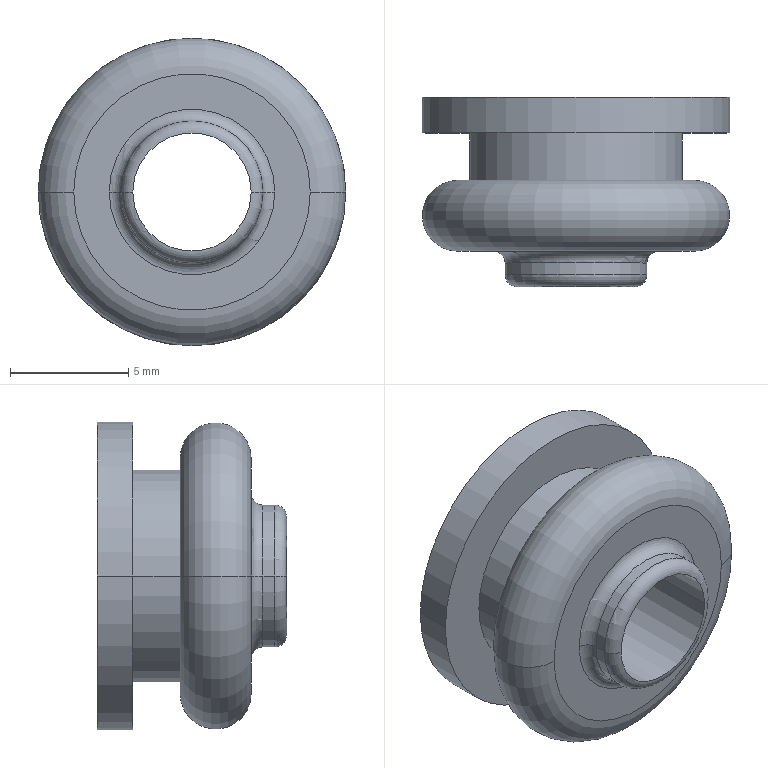Part | STEP file | 233_07_060_230 | 1 solid | 18 faces | box 13 x 8 x 13 mm | volume 572.53 mm3 | cylinder 8 | torus 6 | plane 4 | commonest cylinder face diameters 5 x2 6 x2 9 x2 13 x2
STEP:
#1=CARTESIAN_POINT('',(0.,0.,0.));
#2=DIRECTION('',(0.,0.,1.));
#3=DIRECTION('',(1.,0.,0.));
#4=AXIS2_PLACEMENT_3D('',#1,#2,#3);
#5=CARTESIAN_POINT('',(-2.5,0.,0.));
#6=VERTEX_POINT('',#5);
#7=CARTESIAN_POINT('',(-2.5,-8.,0.));
#8=VERTEX_POINT('',#7);
#9=CARTESIAN_POINT('',(-2.5,0.,0.));
#10=DIRECTION('',(0.,-1.,0.));
#11=VECTOR('',#10,1.);
#12=LINE('',#9,#11);
#13=CARTESIAN_POINT('',(0.,0.4,0.));
#14=DIRECTION('',(0.,-1.,0.));
#15=DIRECTION('',(1.,0.,0.));
#16=AXIS2_PLACEMENT_3D('',#13,#14,#15);
#17=CYLINDRICAL_SURFACE('',#16,2.5);
#18=CARTESIAN_POINT('',(3.142,0.4));
#19=DIRECTION('',(0.,1.));
#20=VECTOR('',#19,1.);
#21=LINE('',#18,#20);
#22=(GEOMETRIC_REPRESENTATION_CONTEXT(2)PARAMETRIC_REPRESENTATION_CONTEXT()REPRESENTATION_CONTEXT('',''));
#23=DEFINITIONAL_REPRESENTATION('',(#21),#22);
#24=PCURVE('',#17,#23);
#25=CARTESIAN_POINT('',(0.,0.4,0.));
#26=DIRECTION('',(0.,-1.,0.));
#27=DIRECTION('',(1.,0.,0.));
#28=AXIS2_PLACEMENT_3D('',#25,#26,#27);
#29=CYLINDRICAL_SURFACE('',#28,2.5);
#30=CARTESIAN_POINT('',(3.142,0.4));
#31=DIRECTION('',(0.,1.));
#32=VECTOR('',#31,1.);
#33=LINE('',#30,#32);
#34=(GEOMETRIC_REPRESENTATION_CONTEXT(2)PARAMETRIC_REPRESENTATION_CONTEXT()REPRESENTATION_CONTEXT('',''));
#35=DEFINITIONAL_REPRESENTATION('',(#33),#34);
#36=PCURVE('',#29,#35);
#37=SURFACE_CURVE('',#12,(#24,#36),.PCURVE_S1.);
#38=EDGE_CURVE('',#6,#8,#37,.T.);
#39=ORIENTED_EDGE('',*,*,#38,.F.);
#40=CARTESIAN_POINT('',(2.5,0.,0.));
#41=VERTEX_POINT('',#40);
#42=CARTESIAN_POINT('',(0.,0.,0.));
#43=DIRECTION('',(0.,-1.,0.));
#44=DIRECTION('',(-1.,0.,0.));
#45=AXIS2_PLACEMENT_3D('',#42,#43,#44);
#46=CIRCLE('',#45,2.5);
#47=CARTESIAN_POINT('',(3.142,0.4));
#48=DIRECTION('',(1.,0.));
#49=VECTOR('',#48,1.);
#50=LINE('',#47,#49);
#51=(GEOMETRIC_REPRESENTATION_CONTEXT(2)PARAMETRIC_REPRESENTATION_CONTEXT()REPRESENTATION_CONTEXT('',''));
#52=DEFINITIONAL_REPRESENTATION('',(#50),#51);
#53=PCURVE('',#17,#52);
#54=CARTESIAN_POINT('',(0.,0.,0.));
#55=DIRECTION('',(0.,-1.,0.));
#56=DIRECTION('',(1.,0.,0.));
#57=AXIS2_PLACEMENT_3D('',#54,#55,#56);
#58=PLANE('',#57);
#59=CARTESIAN_POINT('',(0.,0.));
#60=DIRECTION('',(-1.,0.));
#61=AXIS2_PLACEMENT_2D('',#59,#60);
#62=CIRCLE('',#61,2.5);
#63=(GEOMETRIC_REPRESENTATION_CONTEXT(2)PARAMETRIC_REPRESENTATION_CONTEXT()REPRESENTATION_CONTEXT('',''));
#64=DEFINITIONAL_REPRESENTATION('',(#62),#63);
#65=PCURVE('',#58,#64);
#66=SURFACE_CURVE('',#46,(#53,#65),.PCURVE_S1.);
#67=EDGE_CURVE('',#6,#41,#66,.T.);
#68=ORIENTED_EDGE('',*,*,#67,.T.);
#69=CARTESIAN_POINT('',(2.5,-8.,0.));
#70=VERTEX_POINT('',#69);
#71=CARTESIAN_POINT('',(2.5,0.,0.));
#72=DIRECTION('',(0.,-1.,0.));
#73=VECTOR('',#72,1.);
#74=LINE('',#71,#73);
#75=CARTESIAN_POINT('',(6.283,0.4));
#76=DIRECTION('',(0.,1.));
#77=VECTOR('',#76,1.);
#78=LINE('',#75,#77);
#79=(GEOMETRIC_REPRESENTATION_CONTEXT(2)PARAMETRIC_REPRESENTATION_CONTEXT()REPRESENTATION_CONTEXT('',''));
#80=DEFINITIONAL_REPRESENTATION('',(#78),#79);
#81=PCURVE('',#17,#80);
#82=CARTESIAN_POINT('',(0.,0.4));
#83=DIRECTION('',(0.,1.));
#84=VECTOR('',#83,1.);
#85=LINE('',#82,#84);
#86=(GEOMETRIC_REPRESENTATION_CONTEXT(2)PARAMETRIC_REPRESENTATION_CONTEXT()REPRESENTATION_CONTEXT('',''));
#87=DEFINITIONAL_REPRESENTATION('',(#85),#86);
#88=PCURVE('',#29,#87);
#89=SURFACE_CURVE('',#74,(#81,#88),.PCURVE_S1.);
#90=EDGE_CURVE('',#41,#70,#89,.T.);
#91=ORIENTED_EDGE('',*,*,#90,.T.);
#92=CARTESIAN_POINT('',(0.,-8.,0.));
#93=DIRECTION('',(0.,-1.,0.));
#94=DIRECTION('',(-1.,0.,0.));
#95=AXIS2_PLACEMENT_3D('',#92,#93,#94);
#96=CIRCLE('',#95,2.5);
#97=CARTESIAN_POINT('',(3.142,8.4));
#98=DIRECTION('',(1.,0.));
#99=VECTOR('',#98,1.);
#100=LINE('',#97,#99);
#101=(GEOMETRIC_REPRESENTATION_CONTEXT(2)PARAMETRIC_REPRESENTATION_CONTEXT()REPRESENTATION_CONTEXT('',''));
#102=DEFINITIONAL_REPRESENTATION('',(#100),#101);
#103=PCURVE('',#17,#102);
#104=CARTESIAN_POINT('',(0.,-7.5,0.));
#105=DIRECTION('',(0.,-1.,0.));
#106=DIRECTION('',(1.,0.,0.));
#107=AXIS2_PLACEMENT_3D('',#104,#105,#106);
#108=TOROIDAL_SURFACE('',#107,2.5,0.5);
#109=CARTESIAN_POINT('',(3.142,1.571));
#110=DIRECTION('',(1.,0.));
#111=VECTOR('',#110,1.);
#112=LINE('',#109,#111);
#113=(GEOMETRIC_REPRESENTATION_CONTEXT(2)PARAMETRIC_REPRESENTATION_CONTEXT()REPRESENTATION_CONTEXT('',''));
#114=DEFINITIONAL_REPRESENTATION('',(#112),#113);
#115=PCURVE('',#108,#114);
#116=SURFACE_CURVE('',#96,(#103,#115),.PCURVE_S1.);
#117=EDGE_CURVE('',#8,#70,#116,.T.);
#118=ORIENTED_EDGE('',*,*,#117,.F.);
#119=EDGE_LOOP('',(#39,#68,#91,#118));
#120=FACE_BOUND('',#119,.F.);
#121=ADVANCED_FACE('',(#120),#17,.F.);
#122=ORIENTED_EDGE('',*,*,#38,.T.);
#123=CARTESIAN_POINT('',(0.,-8.,0.));
#124=DIRECTION('',(0.,1.,0.));
#125=DIRECTION('',(-1.,0.,0.));
#126=AXIS2_PLACEMENT_3D('',#123,#124,#125);
#127=CIRCLE('',#126,2.5);
#128=CARTESIAN_POINT('',(3.142,8.4));
#129=DIRECTION('',(-1.,0.));
#130=VECTOR('',#129,1.);
#131=LINE('',#128,#130);
#132=(GEOMETRIC_REPRESENTATION_CONTEXT(2)PARAMETRIC_REPRESENTATION_CONTEXT()REPRESENTATION_CONTEXT('',''));
#133=DEFINITIONAL_REPRESENTATION('',(#131),#132);
#134=PCURVE('',#29,#133);
#135=CARTESIAN_POINT('',(0.,-7.5,0.));
#136=DIRECTION('',(0.,-1.,0.));
#137=DIRECTION('',(1.,0.,0.));
#138=AXIS2_PLACEMENT_3D('',#135,#136,#137);
#139=TOROIDAL_SURFACE('',#138,2.5,0.5);
#140=CARTESIAN_POINT('',(3.142,1.571));
#141=DIRECTION('',(-1.,0.));
#142=VECTOR('',#141,1.);
#143=LINE('',#140,#142);
#144=(GEOMETRIC_REPRESENTATION_CONTEXT(2)PARAMETRIC_REPRESENTATION_CONTEXT()REPRESENTATION_CONTEXT('',''));
#145=DEFINITIONAL_REPRESENTATION('',(#143),#144);
#146=PCURVE('',#139,#145);
#147=SURFACE_CURVE('',#127,(#134,#146),.PCURVE_S1.);
#148=EDGE_CURVE('',#8,#70,#147,.T.);
#149=ORIENTED_EDGE('',*,*,#148,.T.);
#150=ORIENTED_EDGE('',*,*,#90,.F.);
#151=CARTESIAN_POINT('',(0.,0.,0.));
#152=DIRECTION('',(0.,1.,0.));
#153=DIRECTION('',(-1.,0.,0.));
#154=AXIS2_PLACEMENT_3D('',#151,#152,#153);
#155=CIRCLE('',#154,2.5);
#156=CARTESIAN_POINT('',(3.142,0.4));
#157=DIRECTION('',(-1.,0.));
#158=VECTOR('',#157,1.);
#159=LINE('',#156,#158);
#160=(GEOMETRIC_REPRESENTATION_CONTEXT(2)PARAMETRIC_REPRESENTATION_CONTEXT()REPRESENTATION_CONTEXT('',''));
#161=DEFINITIONAL_REPRESENTATION('',(#159),#160);
#162=PCURVE('',#29,#161);
#163=CARTESIAN_POINT('',(-2.5,0.));
#164=CARTESIAN_POINT('',(-2.5,4.33));
#165=CARTESIAN_POINT('',(1.25,2.165));
#166=CARTESIAN_POINT('',(5.,0.));
#167=CARTESIAN_POINT('',(1.25,-2.165));
#168=CARTESIAN_POINT('',(-2.5,-4.33));
#169=CARTESIAN_POINT('',(-2.5,0.));
#170=(BOUNDED_CURVE()B_SPLINE_CURVE(2,(#163,#164,#165,#166,#167,#168,#169),.UNSPECIFIED.,.T.,.F.)B_SPLINE_CURVE_WITH_KNOTS((1,2,2,2,2,1),(-2.094,0.,2.094,4.189,6.283,8.378),.UNSPECIFIED.)CURVE()GEOMETRIC_REPRESENTATION_ITEM()RATIONAL_B_SPLINE_CURVE((1.,0.5,1.,0.5,1.,0.5,1.))REPRESENTATION_ITEM(''));
#171=(GEOMETRIC_REPRESENTATION_CONTEXT(2)PARAMETRIC_REPRESENTATION_CONTEXT()REPRESENTATION_CONTEXT('',''));
#172=DEFINITIONAL_REPRESENTATION('',(#170),#171);
#173=PCURVE('',#58,#172);
#174=SURFACE_CURVE('',#155,(#162,#173),.PCURVE_S1.);
#175=EDGE_CURVE('',#6,#41,#174,.T.);
#176=ORIENTED_EDGE('',*,*,#175,.F.);
#177=EDGE_LOOP('',(#122,#149,#150,#176));
#178=FACE_BOUND('',#177,.F.);
#179=ADVANCED_FACE('',(#178),#29,.F.);
#180=ORIENTED_EDGE('',*,*,#148,.T.);
#181=CARTESIAN_POINT('',(3.,-7.5,0.));
#182=VERTEX_POINT('',#181);
#183=CARTESIAN_POINT('',(2.5,-7.5,0.));
#184=DIRECTION('',(0.,0.,1.));
#185=DIRECTION('',(0.,-1.,0.));
#186=AXIS2_PLACEMENT_3D('',#183,#184,#185);
#187=CIRCLE('',#186,0.5);
#188=CARTESIAN_POINT('',(0.,1.571));
#189=DIRECTION('',(0.,-1.));
#190=VECTOR('',#189,1.);
#191=LINE('',#188,#190);
#192=(GEOMETRIC_REPRESENTATION_CONTEXT(2)PARAMETRIC_REPRESENTATION_CONTEXT()REPRESENTATION_CONTEXT('',''));
#193=DEFINITIONAL_REPRESENTATION('',(#191),#192);
#194=PCURVE('',#139,#193);
#195=CARTESIAN_POINT('',(6.283,1.571));
#196=DIRECTION('',(0.,-1.));
#197=VECTOR('',#196,1.);
#198=LINE('',#195,#197);
#199=(GEOMETRIC_REPRESENTATION_CONTEXT(2)PARAMETRIC_REPRESENTATION_CONTEXT()REPRESENTATION_CONTEXT('',''));
#200=DEFINITIONAL_REPRESENTATION('',(#198),#199);
#201=PCURVE('',#108,#200);
#202=SURFACE_CURVE('',#187,(#194,#201),.PCURVE_S1.);
#203=EDGE_CURVE('',#70,#182,#202,.T.);
#204=ORIENTED_EDGE('',*,*,#203,.T.);
#205=CARTESIAN_POINT('',(-3.,-7.5,0.));
#206=VERTEX_POINT('',#205);
#207=CARTESIAN_POINT('',(0.,-7.5,0.));
#208=DIRECTION('',(0.,1.,0.));
#209=DIRECTION('',(-1.,0.,0.));
#210=AXIS2_PLACEMENT_3D('',#207,#208,#209);
#211=CIRCLE('',#210,3.);
#212=CARTESIAN_POINT('',(3.142,0.));
#213=DIRECTION('',(-1.,0.));
#214=VECTOR('',#213,1.);
#215=LINE('',#212,#214);
#216=(GEOMETRIC_REPRESENTATION_CONTEXT(2)PARAMETRIC_REPRESENTATION_CONTEXT()REPRESENTATION_CONTEXT('',''));
#217=DEFINITIONAL_REPRESENTATION('',(#215),#216);
#218=PCURVE('',#139,#217);
#219=CARTESIAN_POINT('',(0.,0.4,0.));
#220=DIRECTION('',(0.,-1.,0.));
#221=DIRECTION('',(1.,0.,0.));
#222=AXIS2_PLACEMENT_3D('',#219,#220,#221);
#223=CYLINDRICAL_SURFACE('',#222,3.);
#224=CARTESIAN_POINT('',(3.142,7.9));
#225=DIRECTION('',(-1.,0.));
#226=VECTOR('',#225,1.);
#227=LINE('',#224,#226);
#228=(GEOMETRIC_REPRESENTATION_CONTEXT(2)PARAMETRIC_REPRESENTATION_CONTEXT()REPRESENTATION_CONTEXT('',''));
#229=DEFINITIONAL_REPRESENTATION('',(#227),#228);
#230=PCURVE('',#223,#229);
#231=SURFACE_CURVE('',#211,(#218,#230),.PCURVE_S1.);
#232=EDGE_CURVE('',#206,#182,#231,.T.);
#233=ORIENTED_EDGE('',*,*,#232,.F.);
#234=CARTESIAN_POINT('',(-2.5,-7.5,0.));
#235=DIRECTION('',(0.,0.,-1.));
#236=DIRECTION('',(0.,-1.,0.));
#237=AXIS2_PLACEMENT_3D('',#234,#235,#236);
#238=CIRCLE('',#237,0.5);
#239=CARTESIAN_POINT('',(3.142,1.571));
#240=DIRECTION('',(0.,-1.));
#241=VECTOR('',#240,1.);
#242=LINE('',#239,#241);
#243=(GEOMETRIC_REPRESENTATION_CONTEXT(2)PARAMETRIC_REPRESENTATION_CONTEXT()REPRESENTATION_CONTEXT('',''));
#244=DEFINITIONAL_REPRESENTATION('',(#242),#243);
#245=PCURVE('',#139,#244);
#246=CARTESIAN_POINT('',(3.142,1.571));
#247=DIRECTION('',(0.,-1.));
#248=VECTOR('',#247,1.);
#249=LINE('',#246,#248);
#250=(GEOMETRIC_REPRESENTATION_CONTEXT(2)PARAMETRIC_REPRESENTATION_CONTEXT()REPRESENTATION_CONTEXT('',''));
#251=DEFINITIONAL_REPRESENTATION('',(#249),#250);
#252=PCURVE('',#108,#251);
#253=SURFACE_CURVE('',#238,(#245,#252),.PCURVE_S1.);
#254=EDGE_CURVE('',#8,#206,#253,.T.);
#255=ORIENTED_EDGE('',*,*,#254,.F.);
#256=EDGE_LOOP('',(#180,#204,#233,#255));
#257=FACE_BOUND('',#256,.T.);
#258=ADVANCED_FACE('',(#257),#139,.T.);
#259=CARTESIAN_POINT('',(0.,-7.5,0.));
#260=DIRECTION('',(0.,-1.,0.));
#261=DIRECTION('',(-1.,0.,0.));
#262=AXIS2_PLACEMENT_3D('',#259,#260,#261);
#263=CIRCLE('',#262,3.);
#264=CARTESIAN_POINT('',(3.142,0.));
#265=DIRECTION('',(1.,0.));
#266=VECTOR('',#265,1.);
#267=LINE('',#264,#266);
#268=(GEOMETRIC_REPRESENTATION_CONTEXT(2)PARAMETRIC_REPRESENTATION_CONTEXT()REPRESENTATION_CONTEXT('',''));
#269=DEFINITIONAL_REPRESENTATION('',(#267),#268);
#270=PCURVE('',#108,#269);
#271=CARTESIAN_POINT('',(0.,0.4,0.));
#272=DIRECTION('',(0.,-1.,0.));
#273=DIRECTION('',(1.,0.,0.));
#274=AXIS2_PLACEMENT_3D('',#271,#272,#273);
#275=CYLINDRICAL_SURFACE('',#274,3.);
#276=CARTESIAN_POINT('',(3.142,7.9));
#277=DIRECTION('',(1.,0.));
#278=VECTOR('',#277,1.);
#279=LINE('',#276,#278);
#280=(GEOMETRIC_REPRESENTATION_CONTEXT(2)PARAMETRIC_REPRESENTATION_CONTEXT()REPRESENTATION_CONTEXT('',''));
#281=DEFINITIONAL_REPRESENTATION('',(#279),#280);
#282=PCURVE('',#275,#281);
#283=SURFACE_CURVE('',#263,(#270,#282),.PCURVE_S1.);
#284=EDGE_CURVE('',#206,#182,#283,.T.);
#285=ORIENTED_EDGE('',*,*,#284,.T.);
#286=ORIENTED_EDGE('',*,*,#203,.F.);
#287=ORIENTED_EDGE('',*,*,#117,.F.);
#288=ORIENTED_EDGE('',*,*,#254,.T.);
#289=EDGE_LOOP('',(#285,#286,#287,#288));
#290=FACE_BOUND('',#289,.T.);
#291=ADVANCED_FACE('',(#290),#108,.T.);
#292=CARTESIAN_POINT('',(-3.,-7.,0.));
#293=VERTEX_POINT('',#292);
#294=CARTESIAN_POINT('',(3.,-7.,0.));
#295=VERTEX_POINT('',#294);
#296=CARTESIAN_POINT('',(0.,-7.,0.));
#297=DIRECTION('',(0.,-1.,0.));
#298=DIRECTION('',(-1.,0.,0.));
#299=AXIS2_PLACEMENT_3D('',#296,#297,#298);
#300=CIRCLE('',#299,3.);
#301=CARTESIAN_POINT('',(3.142,7.4));
#302=DIRECTION('',(1.,0.));
#303=VECTOR('',#302,1.);
#304=LINE('',#301,#303);
#305=(GEOMETRIC_REPRESENTATION_CONTEXT(2)PARAMETRIC_REPRESENTATION_CONTEXT()REPRESENTATION_CONTEXT('',''));
#306=DEFINITIONAL_REPRESENTATION('',(#304),#305);
#307=PCURVE('',#275,#306);
#308=CARTESIAN_POINT('',(0.,-7.,0.));
#309=DIRECTION('',(0.,-1.,0.));
#310=DIRECTION('',(1.,0.,0.));
#311=AXIS2_PLACEMENT_3D('',#308,#309,#310);
#312=TOROIDAL_SURFACE('',#311,3.5,0.5);
#313=CARTESIAN_POINT('',(3.142,3.142));
#314=DIRECTION('',(1.,0.));
#315=VECTOR('',#314,1.);
#316=LINE('',#313,#315);
#317=(GEOMETRIC_REPRESENTATION_CONTEXT(2)PARAMETRIC_REPRESENTATION_CONTEXT()REPRESENTATION_CONTEXT('',''));
#318=DEFINITIONAL_REPRESENTATION('',(#316),#317);
#319=PCURVE('',#312,#318);
#320=SURFACE_CURVE('',#300,(#307,#319),.PCURVE_S1.);
#321=EDGE_CURVE('',#293,#295,#320,.T.);
#322=ORIENTED_EDGE('',*,*,#321,.T.);
#323=CARTESIAN_POINT('',(3.,-7.5,0.));
#324=DIRECTION('',(0.,1.,0.));
#325=VECTOR('',#324,1.);
#326=LINE('',#323,#325);
#327=CARTESIAN_POINT('',(6.283,7.9));
#328=DIRECTION('',(0.,-1.));
#329=VECTOR('',#328,1.);
#330=LINE('',#327,#329);
#331=(GEOMETRIC_REPRESENTATION_CONTEXT(2)PARAMETRIC_REPRESENTATION_CONTEXT()REPRESENTATION_CONTEXT('',''));
#332=DEFINITIONAL_REPRESENTATION('',(#330),#331);
#333=PCURVE('',#275,#332);
#334=CARTESIAN_POINT('',(0.,7.9));
#335=DIRECTION('',(0.,-1.));
#336=VECTOR('',#335,1.);
#337=LINE('',#334,#336);
#338=(GEOMETRIC_REPRESENTATION_CONTEXT(2)PARAMETRIC_REPRESENTATION_CONTEXT()REPRESENTATION_CONTEXT('',''));
#339=DEFINITIONAL_REPRESENTATION('',(#337),#338);
#340=PCURVE('',#223,#339);
#341=SURFACE_CURVE('',#326,(#333,#340),.PCURVE_S1.);
#342=EDGE_CURVE('',#182,#295,#341,.T.);
#343=ORIENTED_EDGE('',*,*,#342,.F.);
#344=ORIENTED_EDGE('',*,*,#284,.F.);
#345=CARTESIAN_POINT('',(-3.,-7.5,0.));
#346=DIRECTION('',(0.,1.,0.));
#347=VECTOR('',#346,1.);
#348=LINE('',#345,#347);
#349=CARTESIAN_POINT('',(3.142,7.9));
#350=DIRECTION('',(0.,-1.));
#351=VECTOR('',#350,1.);
#352=LINE('',#349,#351);
#353=(GEOMETRIC_REPRESENTATION_CONTEXT(2)PARAMETRIC_REPRESENTATION_CONTEXT()REPRESENTATION_CONTEXT('',''));
#354=DEFINITIONAL_REPRESENTATION('',(#352),#353);
#355=PCURVE('',#275,#354);
#356=CARTESIAN_POINT('',(3.142,7.9));
#357=DIRECTION('',(0.,-1.));
#358=VECTOR('',#357,1.);
#359=LINE('',#356,#358);
#360=(GEOMETRIC_REPRESENTATION_CONTEXT(2)PARAMETRIC_REPRESENTATION_CONTEXT()REPRESENTATION_CONTEXT('',''));
#361=DEFINITIONAL_REPRESENTATION('',(#359),#360);
#362=PCURVE('',#223,#361);
#363=SURFACE_CURVE('',#348,(#355,#362),.PCURVE_S1.);
#364=EDGE_CURVE('',#206,#293,#363,.T.);
#365=ORIENTED_EDGE('',*,*,#364,.T.);
#366=EDGE_LOOP('',(#322,#343,#344,#365));
#367=FACE_BOUND('',#366,.T.);
#368=ADVANCED_FACE('',(#367),#275,.T.);
#369=ORIENTED_EDGE('',*,*,#232,.T.);
#370=ORIENTED_EDGE('',*,*,#342,.T.);
#371=CARTESIAN_POINT('',(0.,-7.,0.));
#372=DIRECTION('',(0.,1.,0.));
#373=DIRECTION('',(-1.,0.,0.));
#374=AXIS2_PLACEMENT_3D('',#371,#372,#373);
#375=CIRCLE('',#374,3.);
#376=CARTESIAN_POINT('',(3.142,7.4));
#377=DIRECTION('',(-1.,0.));
#378=VECTOR('',#377,1.);
#379=LINE('',#376,#378);
#380=(GEOMETRIC_REPRESENTATION_CONTEXT(2)PARAMETRIC_REPRESENTATION_CONTEXT()REPRESENTATION_CONTEXT('',''));
#381=DEFINITIONAL_REPRESENTATION('',(#379),#380);
#382=PCURVE('',#223,#381);
#383=CARTESIAN_POINT('',(0.,-7.,0.));
#384=DIRECTION('',(0.,-1.,0.));
#385=DIRECTION('',(1.,0.,0.));
#386=AXIS2_PLACEMENT_3D('',#383,#384,#385);
#387=TOROIDAL_SURFACE('',#386,3.5,0.5);
#388=CARTESIAN_POINT('',(3.142,3.142));
#389=DIRECTION('',(-1.,0.));
#390=VECTOR('',#389,1.);
#391=LINE('',#388,#390);
#392=(GEOMETRIC_REPRESENTATION_CONTEXT(2)PARAMETRIC_REPRESENTATION_CONTEXT()REPRESENTATION_CONTEXT('',''));
#393=DEFINITIONAL_REPRESENTATION('',(#391),#392);
#394=PCURVE('',#387,#393);
#395=SURFACE_CURVE('',#375,(#382,#394),.PCURVE_S1.);
#396=EDGE_CURVE('',#293,#295,#395,.T.);
#397=ORIENTED_EDGE('',*,*,#396,.F.);
#398=ORIENTED_EDGE('',*,*,#364,.F.);
#399=EDGE_LOOP('',(#369,#370,#397,#398));
#400=FACE_BOUND('',#399,.T.);
#401=ADVANCED_FACE('',(#400),#223,.T.);
#402=CARTESIAN_POINT('',(-3.5,-6.5,0.));
#403=VERTEX_POINT('',#402);
#404=CARTESIAN_POINT('',(-3.5,-7.,0.));
#405=DIRECTION('',(0.,0.,1.));
#406=DIRECTION('',(1.,0.,0.));
#407=AXIS2_PLACEMENT_3D('',#404,#405,#406);
#408=CIRCLE('',#407,0.5);
#409=CARTESIAN_POINT('',(3.142,3.142));
#410=DIRECTION('',(0.,1.));
#411=VECTOR('',#410,1.);
#412=LINE('',#409,#411);
#413=(GEOMETRIC_REPRESENTATION_CONTEXT(2)PARAMETRIC_REPRESENTATION_CONTEXT()REPRESENTATION_CONTEXT('',''));
#414=DEFINITIONAL_REPRESENTATION('',(#412),#413);
#415=PCURVE('',#387,#414);
#416=CARTESIAN_POINT('',(3.142,3.142));
#417=DIRECTION('',(0.,1.));
#418=VECTOR('',#417,1.);
#419=LINE('',#416,#418);
#420=(GEOMETRIC_REPRESENTATION_CONTEXT(2)PARAMETRIC_REPRESENTATION_CONTEXT()REPRESENTATION_CONTEXT('',''));
#421=DEFINITIONAL_REPRESENTATION('',(#419),#420);
#422=PCURVE('',#312,#421);
#423=SURFACE_CURVE('',#408,(#415,#422),.PCURVE_S1.);
#424=EDGE_CURVE('',#293,#403,#423,.T.);
#425=ORIENTED_EDGE('',*,*,#424,.T.);
#426=CARTESIAN_POINT('',(3.5,-6.5,0.));
#427=VERTEX_POINT('',#426);
#428=CARTESIAN_POINT('',(0.,-6.5,0.));
#429=DIRECTION('',(0.,1.,0.));
#430=DIRECTION('',(-1.,0.,0.));
#431=AXIS2_PLACEMENT_3D('',#428,#429,#430);
#432=CIRCLE('',#431,3.5);
#433=CARTESIAN_POINT('',(3.142,4.712));
#434=DIRECTION('',(-1.,0.));
#435=VECTOR('',#434,1.);
#436=LINE('',#433,#435);
#437=(GEOMETRIC_REPRESENTATION_CONTEXT(2)PARAMETRIC_REPRESENTATION_CONTEXT()REPRESENTATION_CONTEXT('',''));
#438=DEFINITIONAL_REPRESENTATION('',(#436),#437);
#439=PCURVE('',#387,#438);
#440=CARTESIAN_POINT('',(0.,-6.5,0.));
#441=DIRECTION('',(0.,-1.,0.));
#442=DIRECTION('',(1.,0.,0.));
#443=AXIS2_PLACEMENT_3D('',#440,#441,#442);
#444=PLANE('',#443);
#445=CARTESIAN_POINT('',(-3.5,0.));
#446=CARTESIAN_POINT('',(-3.5,6.062));
#447=CARTESIAN_POINT('',(1.75,3.031));
#448=CARTESIAN_POINT('',(7.,0.));
#449=CARTESIAN_POINT('',(1.75,-3.031));
#450=CARTESIAN_POINT('',(-3.5,-6.062));
#451=CARTESIAN_POINT('',(-3.5,0.));
#452=(BOUNDED_CURVE()B_SPLINE_CURVE(2,(#445,#446,#447,#448,#449,#450,#451),.UNSPECIFIED.,.T.,.F.)B_SPLINE_CURVE_WITH_KNOTS((1,2,2,2,2,1),(-2.094,0.,2.094,4.189,6.283,8.378),.UNSPECIFIED.)CURVE()GEOMETRIC_REPRESENTATION_ITEM()RATIONAL_B_SPLINE_CURVE((1.,0.5,1.,0.5,1.,0.5,1.))REPRESENTATION_ITEM(''));
#453=(GEOMETRIC_REPRESENTATION_CONTEXT(2)PARAMETRIC_REPRESENTATION_CONTEXT()REPRESENTATION_CONTEXT('',''));
#454=DEFINITIONAL_REPRESENTATION('',(#452),#453);
#455=PCURVE('',#444,#454);
#456=SURFACE_CURVE('',#432,(#439,#455),.PCURVE_S1.);
#457=EDGE_CURVE('',#403,#427,#456,.T.);
#458=ORIENTED_EDGE('',*,*,#457,.T.);
#459=CARTESIAN_POINT('',(3.5,-7.,0.));
#460=DIRECTION('',(0.,0.,-1.));
#461=DIRECTION('',(-1.,0.,0.));
#462=AXIS2_PLACEMENT_3D('',#459,#460,#461);
#463=CIRCLE('',#462,0.5);
#464=CARTESIAN_POINT('',(0.,3.142));
#465=DIRECTION('',(0.,1.));
#466=VECTOR('',#465,1.);
#467=LINE('',#464,#466);
#468=(GEOMETRIC_REPRESENTATION_CONTEXT(2)PARAMETRIC_REPRESENTATION_CONTEXT()REPRESENTATION_CONTEXT('',''));
#469=DEFINITIONAL_REPRESENTATION('',(#467),#468);
#470=PCURVE('',#387,#469);
#471=CARTESIAN_POINT('',(6.283,3.142));
#472=DIRECTION('',(0.,1.));
#473=VECTOR('',#472,1.);
#474=LINE('',#471,#473);
#475=(GEOMETRIC_REPRESENTATION_CONTEXT(2)PARAMETRIC_REPRESENTATION_CONTEXT()REPRESENTATION_CONTEXT('',''));
#476=DEFINITIONAL_REPRESENTATION('',(#474),#475);
#477=PCURVE('',#312,#476);
#478=SURFACE_CURVE('',#463,(#470,#477),.PCURVE_S1.);
#479=EDGE_CURVE('',#295,#427,#478,.T.);
#480=ORIENTED_EDGE('',*,*,#479,.F.);
#481=ORIENTED_EDGE('',*,*,#396,.F.);
#482=EDGE_LOOP('',(#425,#458,#480,#481));
#483=FACE_BOUND('',#482,.F.);
#484=ADVANCED_FACE('',(#483),#387,.F.);
#485=ORIENTED_EDGE('',*,*,#424,.F.);
#486=ORIENTED_EDGE('',*,*,#321,.T.);
#487=ORIENTED_EDGE('',*,*,#479,.T.);
#488=CARTESIAN_POINT('',(0.,-6.5,0.));
#489=DIRECTION('',(0.,-1.,0.));
#490=DIRECTION('',(-1.,0.,0.));
#491=AXIS2_PLACEMENT_3D('',#488,#489,#490);
#492=CIRCLE('',#491,3.5);
#493=CARTESIAN_POINT('',(3.142,4.712));
#494=DIRECTION('',(1.,0.));
#495=VECTOR('',#494,1.);
#496=LINE('',#493,#495);
#497=(GEOMETRIC_REPRESENTATION_CONTEXT(2)PARAMETRIC_REPRESENTATION_CONTEXT()REPRESENTATION_CONTEXT('',''));
#498=DEFINITIONAL_REPRESENTATION('',(#496),#497);
#499=PCURVE('',#312,#498);
#500=CARTESIAN_POINT('',(0.,0.));
#501=DIRECTION('',(-1.,0.));
#502=AXIS2_PLACEMENT_2D('',#500,#501);
#503=CIRCLE('',#502,3.5);
#504=(GEOMETRIC_REPRESENTATION_CONTEXT(2)PARAMETRIC_REPRESENTATION_CONTEXT()REPRESENTATION_CONTEXT('',''));
#505=DEFINITIONAL_REPRESENTATION('',(#503),#504);
#506=PCURVE('',#444,#505);
#507=SURFACE_CURVE('',#492,(#499,#506),.PCURVE_S1.);
#508=EDGE_CURVE('',#403,#427,#507,.T.);
#509=ORIENTED_EDGE('',*,*,#508,.F.);
#510=EDGE_LOOP('',(#485,#486,#487,#509));
#511=FACE_BOUND('',#510,.F.);
#512=ADVANCED_FACE('',(#511),#312,.F.);
#513=CARTESIAN_POINT('',(-5.,-6.5,0.));
#514=VERTEX_POINT('',#513);
#515=CARTESIAN_POINT('',(5.,-6.5,0.));
#516=VERTEX_POINT('',#515);
#517=CARTESIAN_POINT('',(0.,-6.5,0.));
#518=DIRECTION('',(0.,-1.,0.));
#519=DIRECTION('',(-1.,0.,0.));
#520=AXIS2_PLACEMENT_3D('',#517,#518,#519);
#521=CIRCLE('',#520,5.);
#522=CARTESIAN_POINT('',(0.,0.));
#523=DIRECTION('',(-1.,0.));
#524=AXIS2_PLACEMENT_2D('',#522,#523);
#525=CIRCLE('',#524,5.);
#526=(GEOMETRIC_REPRESENTATION_CONTEXT(2)PARAMETRIC_REPRESENTATION_CONTEXT()REPRESENTATION_CONTEXT('',''));
#527=DEFINITIONAL_REPRESENTATION('',(#525),#526);
#528=PCURVE('',#444,#527);
#529=CARTESIAN_POINT('',(0.,-5.,0.));
#530=DIRECTION('',(0.,-1.,0.));
#531=DIRECTION('',(1.,0.,0.));
#532=AXIS2_PLACEMENT_3D('',#529,#530,#531);
#533=TOROIDAL_SURFACE('',#532,5.,1.5);
#534=CARTESIAN_POINT('',(3.142,7.854));
#535=DIRECTION('',(1.,0.));
#536=VECTOR('',#535,1.);
#537=LINE('',#534,#536);
#538=(GEOMETRIC_REPRESENTATION_CONTEXT(2)PARAMETRIC_REPRESENTATION_CONTEXT()REPRESENTATION_CONTEXT('',''));
#539=DEFINITIONAL_REPRESENTATION('',(#537),#538);
#540=PCURVE('',#533,#539);
#541=SURFACE_CURVE('',#521,(#528,#540),.PCURVE_S1.);
#542=EDGE_CURVE('',#514,#516,#541,.T.);
#543=ORIENTED_EDGE('',*,*,#542,.F.);
#544=CARTESIAN_POINT('',(0.,-6.5,0.));
#545=DIRECTION('',(0.,1.,0.));
#546=DIRECTION('',(-1.,0.,0.));
#547=AXIS2_PLACEMENT_3D('',#544,#545,#546);
#548=CIRCLE('',#547,5.);
#549=CARTESIAN_POINT('',(-5.,0.));
#550=CARTESIAN_POINT('',(-5.,8.66));
#551=CARTESIAN_POINT('',(2.5,4.33));
#552=CARTESIAN_POINT('',(10.,0.));
#553=CARTESIAN_POINT('',(2.5,-4.33));
#554=CARTESIAN_POINT('',(-5.,-8.66));
#555=CARTESIAN_POINT('',(-5.,0.));
#556=(BOUNDED_CURVE()B_SPLINE_CURVE(2,(#549,#550,#551,#552,#553,#554,#555),.UNSPECIFIED.,.T.,.F.)B_SPLINE_CURVE_WITH_KNOTS((1,2,2,2,2,1),(-2.094,0.,2.094,4.189,6.283,8.378),.UNSPECIFIED.)CURVE()GEOMETRIC_REPRESENTATION_ITEM()RATIONAL_B_SPLINE_CURVE((1.,0.5,1.,0.5,1.,0.5,1.))REPRESENTATION_ITEM(''));
#557=(GEOMETRIC_REPRESENTATION_CONTEXT(2)PARAMETRIC_REPRESENTATION_CONTEXT()REPRESENTATION_CONTEXT('',''));
#558=DEFINITIONAL_REPRESENTATION('',(#556),#557);
#559=PCURVE('',#444,#558);
#560=CARTESIAN_POINT('',(0.,-5.,0.));
#561=DIRECTION('',(0.,-1.,0.));
#562=DIRECTION('',(1.,0.,0.));
#563=AXIS2_PLACEMENT_3D('',#560,#561,#562);
#564=TOROIDAL_SURFACE('',#563,5.,1.5);
#565=CARTESIAN_POINT('',(3.142,1.571));
#566=DIRECTION('',(-1.,0.));
#567=VECTOR('',#566,1.);
#568=LINE('',#565,#567);
#569=(GEOMETRIC_REPRESENTATION_CONTEXT(2)PARAMETRIC_REPRESENTATION_CONTEXT()REPRESENTATION_CONTEXT('',''));
#570=DEFINITIONAL_REPRESENTATION('',(#568),#569);
#571=PCURVE('',#564,#570);
#572=SURFACE_CURVE('',#548,(#559,#571),.PCURVE_S1.);
#573=EDGE_CURVE('',#514,#516,#572,.T.);
#574=ORIENTED_EDGE('',*,*,#573,.T.);
#575=EDGE_LOOP('',(#543,#574));
#576=FACE_BOUND('',#575,.F.);
#577=ORIENTED_EDGE('',*,*,#457,.F.);
#578=ORIENTED_EDGE('',*,*,#508,.T.);
#579=EDGE_LOOP('',(#577,#578));
#580=FACE_BOUND('',#579,.F.);
#581=ADVANCED_FACE('',(#576,#580),#444,.T.);
#582=CARTESIAN_POINT('',(-5.,-3.5,0.));
#583=VERTEX_POINT('',#582);
#584=CARTESIAN_POINT('',(5.,-3.5,0.));
#585=VERTEX_POINT('',#584);
#586=CARTESIAN_POINT('',(0.,-3.5,0.));
#587=DIRECTION('',(0.,-1.,0.));
#588=DIRECTION('',(-1.,0.,0.));
#589=AXIS2_PLACEMENT_3D('',#586,#587,#588);
#590=CIRCLE('',#589,5.);
#591=CARTESIAN_POINT('',(3.142,4.712));
#592=DIRECTION('',(1.,0.));
#593=VECTOR('',#592,1.);
#594=LINE('',#591,#593);
#595=(GEOMETRIC_REPRESENTATION_CONTEXT(2)PARAMETRIC_REPRESENTATION_CONTEXT()REPRESENTATION_CONTEXT('',''));
#596=DEFINITIONAL_REPRESENTATION('',(#594),#595);
#597=PCURVE('',#533,#596);
#598=CARTESIAN_POINT('',(0.,-3.5,0.));
#599=DIRECTION('',(0.,-1.,0.));
#600=DIRECTION('',(1.,0.,0.));
#601=AXIS2_PLACEMENT_3D('',#598,#599,#600);
#602=PLANE('',#601);
#603=CARTESIAN_POINT('',(0.,0.));
#604=DIRECTION('',(-1.,0.));
#605=AXIS2_PLACEMENT_2D('',#603,#604);
#606=CIRCLE('',#605,5.);
#607=(GEOMETRIC_REPRESENTATION_CONTEXT(2)PARAMETRIC_REPRESENTATION_CONTEXT()REPRESENTATION_CONTEXT('',''));
#608=DEFINITIONAL_REPRESENTATION('',(#606),#607);
#609=PCURVE('',#602,#608);
#610=SURFACE_CURVE('',#590,(#597,#609),.PCURVE_S1.);
#611=EDGE_CURVE('',#583,#585,#610,.T.);
#612=ORIENTED_EDGE('',*,*,#611,.T.);
#613=CARTESIAN_POINT('',(5.,-5.,0.));
#614=DIRECTION('',(0.,0.,1.));
#615=DIRECTION('',(0.,-1.,0.));
#616=AXIS2_PLACEMENT_3D('',#613,#614,#615);
#617=CIRCLE('',#616,1.5);
#618=CARTESIAN_POINT('',(6.283,7.854));
#619=DIRECTION('',(0.,-1.));
#620=VECTOR('',#619,1.);
#621=LINE('',#618,#620);
#622=(GEOMETRIC_REPRESENTATION_CONTEXT(2)PARAMETRIC_REPRESENTATION_CONTEXT()REPRESENTATION_CONTEXT('',''));
#623=DEFINITIONAL_REPRESENTATION('',(#621),#622);
#624=PCURVE('',#533,#623);
#625=CARTESIAN_POINT('',(0.,1.571));
#626=DIRECTION('',(0.,-1.));
#627=VECTOR('',#626,1.);
#628=LINE('',#625,#627);
#629=(GEOMETRIC_REPRESENTATION_CONTEXT(2)PARAMETRIC_REPRESENTATION_CONTEXT()REPRESENTATION_CONTEXT('',''));
#630=DEFINITIONAL_REPRESENTATION('',(#628),#629);
#631=PCURVE('',#564,#630);
#632=SURFACE_CURVE('',#617,(#624,#631),.PCURVE_S1.);
#633=EDGE_CURVE('',#516,#585,#632,.T.);
#634=ORIENTED_EDGE('',*,*,#633,.F.);
#635=ORIENTED_EDGE('',*,*,#542,.F.);
#636=CARTESIAN_POINT('',(-5.,-5.,0.));
#637=DIRECTION('',(0.,0.,-1.));
#638=DIRECTION('',(0.,-1.,0.));
#639=AXIS2_PLACEMENT_3D('',#636,#637,#638);
#640=CIRCLE('',#639,1.5);
#641=CARTESIAN_POINT('',(3.142,7.854));
#642=DIRECTION('',(0.,-1.));
#643=VECTOR('',#642,1.);
#644=LINE('',#641,#643);
#645=(GEOMETRIC_REPRESENTATION_CONTEXT(2)PARAMETRIC_REPRESENTATION_CONTEXT()REPRESENTATION_CONTEXT('',''));
#646=DEFINITIONAL_REPRESENTATION('',(#644),#645);
#647=PCURVE('',#533,#646);
#648=CARTESIAN_POINT('',(3.142,1.571));
#649=DIRECTION('',(0.,-1.));
#650=VECTOR('',#649,1.);
#651=LINE('',#648,#650);
#652=(GEOMETRIC_REPRESENTATION_CONTEXT(2)PARAMETRIC_REPRESENTATION_CONTEXT()REPRESENTATION_CONTEXT('',''));
#653=DEFINITIONAL_REPRESENTATION('',(#651),#652);
#654=PCURVE('',#564,#653);
#655=SURFACE_CURVE('',#640,(#647,#654),.PCURVE_S1.);
#656=EDGE_CURVE('',#514,#583,#655,.T.);
#657=ORIENTED_EDGE('',*,*,#656,.T.);
#658=EDGE_LOOP('',(#612,#634,#635,#657));
#659=FACE_BOUND('',#658,.T.);
#660=ADVANCED_FACE('',(#659),#533,.T.);
#661=ORIENTED_EDGE('',*,*,#573,.T.);
#662=ORIENTED_EDGE('',*,*,#633,.T.);
#663=CARTESIAN_POINT('',(0.,-3.5,0.));
#664=DIRECTION('',(0.,1.,0.));
#665=DIRECTION('',(-1.,0.,0.));
#666=AXIS2_PLACEMENT_3D('',#663,#664,#665);
#667=CIRCLE('',#666,5.);
#668=CARTESIAN_POINT('',(3.142,-1.571));
#669=DIRECTION('',(-1.,0.));
#670=VECTOR('',#669,1.);
#671=LINE('',#668,#670);
#672=(GEOMETRIC_REPRESENTATION_CONTEXT(2)PARAMETRIC_REPRESENTATION_CONTEXT()REPRESENTATION_CONTEXT('',''));
#673=DEFINITIONAL_REPRESENTATION('',(#671),#672);
#674=PCURVE('',#564,#673);
#675=CARTESIAN_POINT('',(-5.,0.));
#676=CARTESIAN_POINT('',(-5.,8.66));
#677=CARTESIAN_POINT('',(2.5,4.33));
#678=CARTESIAN_POINT('',(10.,0.));
#679=CARTESIAN_POINT('',(2.5,-4.33));
#680=CARTESIAN_POINT('',(-5.,-8.66));
#681=CARTESIAN_POINT('',(-5.,0.));
#682=(BOUNDED_CURVE()B_SPLINE_CURVE(2,(#675,#676,#677,#678,#679,#680,#681),.UNSPECIFIED.,.T.,.F.)B_SPLINE_CURVE_WITH_KNOTS((1,2,2,2,2,1),(-2.094,0.,2.094,4.189,6.283,8.378),.UNSPECIFIED.)CURVE()GEOMETRIC_REPRESENTATION_ITEM()RATIONAL_B_SPLINE_CURVE((1.,0.5,1.,0.5,1.,0.5,1.))REPRESENTATION_ITEM(''));
#683=(GEOMETRIC_REPRESENTATION_CONTEXT(2)PARAMETRIC_REPRESENTATION_CONTEXT()REPRESENTATION_CONTEXT('',''));
#684=DEFINITIONAL_REPRESENTATION('',(#682),#683);
#685=PCURVE('',#602,#684);
#686=SURFACE_CURVE('',#667,(#674,#685),.PCURVE_S1.);
#687=EDGE_CURVE('',#583,#585,#686,.T.);
#688=ORIENTED_EDGE('',*,*,#687,.F.);
#689=ORIENTED_EDGE('',*,*,#656,.F.);
#690=EDGE_LOOP('',(#661,#662,#688,#689));
#691=FACE_BOUND('',#690,.T.);
#692=ADVANCED_FACE('',(#691),#564,.T.);
#693=ORIENTED_EDGE('',*,*,#687,.F.);
#694=ORIENTED_EDGE('',*,*,#611,.T.);
#695=EDGE_LOOP('',(#693,#694));
#696=FACE_BOUND('',#695,.F.);
#697=CARTESIAN_POINT('',(-4.5,-3.5,0.));
#698=VERTEX_POINT('',#697);
#699=CARTESIAN_POINT('',(4.5,-3.5,0.));
#700=VERTEX_POINT('',#699);
#701=CARTESIAN_POINT('',(0.,-3.5,0.));
#702=DIRECTION('',(0.,-1.,0.));
#703=DIRECTION('',(-1.,0.,0.));
#704=AXIS2_PLACEMENT_3D('',#701,#702,#703);
#705=CIRCLE('',#704,4.5);
#706=CARTESIAN_POINT('',(0.,0.));
#707=DIRECTION('',(-1.,0.));
#708=AXIS2_PLACEMENT_2D('',#706,#707);
#709=CIRCLE('',#708,4.5);
#710=(GEOMETRIC_REPRESENTATION_CONTEXT(2)PARAMETRIC_REPRESENTATION_CONTEXT()REPRESENTATION_CONTEXT('',''));
#711=DEFINITIONAL_REPRESENTATION('',(#709),#710);
#712=PCURVE('',#602,#711);
#713=CARTESIAN_POINT('',(0.,0.4,0.));
#714=DIRECTION('',(0.,-1.,0.));
#715=DIRECTION('',(1.,0.,0.));
#716=AXIS2_PLACEMENT_3D('',#713,#714,#715);
#717=CYLINDRICAL_SURFACE('',#716,4.5);
#718=CARTESIAN_POINT('',(3.142,3.9));
#719=DIRECTION('',(1.,0.));
#720=VECTOR('',#719,1.);
#721=LINE('',#718,#720);
#722=(GEOMETRIC_REPRESENTATION_CONTEXT(2)PARAMETRIC_REPRESENTATION_CONTEXT()REPRESENTATION_CONTEXT('',''));
#723=DEFINITIONAL_REPRESENTATION('',(#721),#722);
#724=PCURVE('',#717,#723);
#725=SURFACE_CURVE('',#705,(#712,#724),.PCURVE_S1.);
#726=EDGE_CURVE('',#698,#700,#725,.T.);
#727=ORIENTED_EDGE('',*,*,#726,.F.);
#728=CARTESIAN_POINT('',(0.,-3.5,0.));
#729=DIRECTION('',(0.,1.,0.));
#730=DIRECTION('',(-1.,0.,0.));
#731=AXIS2_PLACEMENT_3D('',#728,#729,#730);
#732=CIRCLE('',#731,4.5);
#733=CARTESIAN_POINT('',(-4.5,0.));
#734=CARTESIAN_POINT('',(-4.5,7.794));
#735=CARTESIAN_POINT('',(2.25,3.897));
#736=CARTESIAN_POINT('',(9.,0.));
#737=CARTESIAN_POINT('',(2.25,-3.897));
#738=CARTESIAN_POINT('',(-4.5,-7.794));
#739=CARTESIAN_POINT('',(-4.5,0.));
#740=(BOUNDED_CURVE()B_SPLINE_CURVE(2,(#733,#734,#735,#736,#737,#738,#739),.UNSPECIFIED.,.T.,.F.)B_SPLINE_CURVE_WITH_KNOTS((1,2,2,2,2,1),(-2.094,0.,2.094,4.189,6.283,8.378),.UNSPECIFIED.)CURVE()GEOMETRIC_REPRESENTATION_ITEM()RATIONAL_B_SPLINE_CURVE((1.,0.5,1.,0.5,1.,0.5,1.))REPRESENTATION_ITEM(''));
#741=(GEOMETRIC_REPRESENTATION_CONTEXT(2)PARAMETRIC_REPRESENTATION_CONTEXT()REPRESENTATION_CONTEXT('',''));
#742=DEFINITIONAL_REPRESENTATION('',(#740),#741);
#743=PCURVE('',#602,#742);
#744=CARTESIAN_POINT('',(0.,0.4,0.));
#745=DIRECTION('',(0.,-1.,0.));
#746=DIRECTION('',(1.,0.,0.));
#747=AXIS2_PLACEMENT_3D('',#744,#745,#746);
#748=CYLINDRICAL_SURFACE('',#747,4.5);
#749=CARTESIAN_POINT('',(3.142,3.9));
#750=DIRECTION('',(-1.,0.));
#751=VECTOR('',#750,1.);
#752=LINE('',#749,#751);
#753=(GEOMETRIC_REPRESENTATION_CONTEXT(2)PARAMETRIC_REPRESENTATION_CONTEXT()REPRESENTATION_CONTEXT('',''));
#754=DEFINITIONAL_REPRESENTATION('',(#752),#753);
#755=PCURVE('',#748,#754);
#756=SURFACE_CURVE('',#732,(#743,#755),.PCURVE_S1.);
#757=EDGE_CURVE('',#698,#700,#756,.T.);
#758=ORIENTED_EDGE('',*,*,#757,.T.);
#759=EDGE_LOOP('',(#727,#758));
#760=FACE_BOUND('',#759,.F.);
#761=ADVANCED_FACE('',(#696,#760),#602,.F.);
#762=CARTESIAN_POINT('',(-4.5,-1.5,0.));
#763=VERTEX_POINT('',#762);
#764=CARTESIAN_POINT('',(4.5,-1.5,0.));
#765=VERTEX_POINT('',#764);
#766=CARTESIAN_POINT('',(0.,-1.5,0.));
#767=DIRECTION('',(0.,-1.,0.));
#768=DIRECTION('',(-1.,0.,0.));
#769=AXIS2_PLACEMENT_3D('',#766,#767,#768);
#770=CIRCLE('',#769,4.5);
#771=CARTESIAN_POINT('',(3.142,1.9));
#772=DIRECTION('',(1.,0.));
#773=VECTOR('',#772,1.);
#774=LINE('',#771,#773);
#775=(GEOMETRIC_REPRESENTATION_CONTEXT(2)PARAMETRIC_REPRESENTATION_CONTEXT()REPRESENTATION_CONTEXT('',''));
#776=DEFINITIONAL_REPRESENTATION('',(#774),#775);
#777=PCURVE('',#717,#776);
#778=CARTESIAN_POINT('',(0.,-1.5,0.));
#779=DIRECTION('',(0.,-1.,0.));
#780=DIRECTION('',(1.,0.,0.));
#781=AXIS2_PLACEMENT_3D('',#778,#779,#780);
#782=PLANE('',#781);
#783=CARTESIAN_POINT('',(0.,0.));
#784=DIRECTION('',(-1.,0.));
#785=AXIS2_PLACEMENT_2D('',#783,#784);
#786=CIRCLE('',#785,4.5);
#787=(GEOMETRIC_REPRESENTATION_CONTEXT(2)PARAMETRIC_REPRESENTATION_CONTEXT()REPRESENTATION_CONTEXT('',''));
#788=DEFINITIONAL_REPRESENTATION('',(#786),#787);
#789=PCURVE('',#782,#788);
#790=SURFACE_CURVE('',#770,(#777,#789),.PCURVE_S1.);
#791=EDGE_CURVE('',#763,#765,#790,.T.);
#792=ORIENTED_EDGE('',*,*,#791,.T.);
#793=CARTESIAN_POINT('',(4.5,-3.5,0.));
#794=DIRECTION('',(0.,1.,0.));
#795=VECTOR('',#794,1.);
#796=LINE('',#793,#795);
#797=CARTESIAN_POINT('',(6.283,3.9));
#798=DIRECTION('',(0.,-1.));
#799=VECTOR('',#798,1.);
#800=LINE('',#797,#799);
#801=(GEOMETRIC_REPRESENTATION_CONTEXT(2)PARAMETRIC_REPRESENTATION_CONTEXT()REPRESENTATION_CONTEXT('',''));
#802=DEFINITIONAL_REPRESENTATION('',(#800),#801);
#803=PCURVE('',#717,#802);
#804=CARTESIAN_POINT('',(0.,3.9));
#805=DIRECTION('',(0.,-1.));
#806=VECTOR('',#805,1.);
#807=LINE('',#804,#806);
#808=(GEOMETRIC_REPRESENTATION_CONTEXT(2)PARAMETRIC_REPRESENTATION_CONTEXT()REPRESENTATION_CONTEXT('',''));
#809=DEFINITIONAL_REPRESENTATION('',(#807),#808);
#810=PCURVE('',#748,#809);
#811=SURFACE_CURVE('',#796,(#803,#810),.PCURVE_S1.);
#812=EDGE_CURVE('',#700,#765,#811,.T.);
#813=ORIENTED_EDGE('',*,*,#812,.F.);
#814=ORIENTED_EDGE('',*,*,#726,.F.);
#815=CARTESIAN_POINT('',(-4.5,-3.5,0.));
#816=DIRECTION('',(0.,1.,0.));
#817=VECTOR('',#816,1.);
#818=LINE('',#815,#817);
#819=CARTESIAN_POINT('',(3.142,3.9));
#820=DIRECTION('',(0.,-1.));
#821=VECTOR('',#820,1.);
#822=LINE('',#819,#821);
#823=(GEOMETRIC_REPRESENTATION_CONTEXT(2)PARAMETRIC_REPRESENTATION_CONTEXT()REPRESENTATION_CONTEXT('',''));
#824=DEFINITIONAL_REPRESENTATION('',(#822),#823);
#825=PCURVE('',#717,#824);
#826=CARTESIAN_POINT('',(3.142,3.9));
#827=DIRECTION('',(0.,-1.));
#828=VECTOR('',#827,1.);
#829=LINE('',#826,#828);
#830=(GEOMETRIC_REPRESENTATION_CONTEXT(2)PARAMETRIC_REPRESENTATION_CONTEXT()REPRESENTATION_CONTEXT('',''));
#831=DEFINITIONAL_REPRESENTATION('',(#829),#830);
#832=PCURVE('',#748,#831);
#833=SURFACE_CURVE('',#818,(#825,#832),.PCURVE_S1.);
#834=EDGE_CURVE('',#698,#763,#833,.T.);
#835=ORIENTED_EDGE('',*,*,#834,.T.);
#836=EDGE_LOOP('',(#792,#813,#814,#835));
#837=FACE_BOUND('',#836,.T.);
#838=ADVANCED_FACE('',(#837),#717,.T.);
#839=ORIENTED_EDGE('',*,*,#757,.T.);
#840=ORIENTED_EDGE('',*,*,#812,.T.);
#841=CARTESIAN_POINT('',(0.,-1.5,0.));
#842=DIRECTION('',(0.,1.,0.));
#843=DIRECTION('',(-1.,0.,0.));
#844=AXIS2_PLACEMENT_3D('',#841,#842,#843);
#845=CIRCLE('',#844,4.5);
#846=CARTESIAN_POINT('',(3.142,1.9));
#847=DIRECTION('',(-1.,0.));
#848=VECTOR('',#847,1.);
#849=LINE('',#846,#848);
#850=(GEOMETRIC_REPRESENTATION_CONTEXT(2)PARAMETRIC_REPRESENTATION_CONTEXT()REPRESENTATION_CONTEXT('',''));
#851=DEFINITIONAL_REPRESENTATION('',(#849),#850);
#852=PCURVE('',#748,#851);
#853=CARTESIAN_POINT('',(-4.5,0.));
#854=CARTESIAN_POINT('',(-4.5,7.794));
#855=CARTESIAN_POINT('',(2.25,3.897));
#856=CARTESIAN_POINT('',(9.,0.));
#857=CARTESIAN_POINT('',(2.25,-3.897));
#858=CARTESIAN_POINT('',(-4.5,-7.794));
#859=CARTESIAN_POINT('',(-4.5,0.));
#860=(BOUNDED_CURVE()B_SPLINE_CURVE(2,(#853,#854,#855,#856,#857,#858,#859),.UNSPECIFIED.,.T.,.F.)B_SPLINE_CURVE_WITH_KNOTS((1,2,2,2,2,1),(-2.094,0.,2.094,4.189,6.283,8.378),.UNSPECIFIED.)CURVE()GEOMETRIC_REPRESENTATION_ITEM()RATIONAL_B_SPLINE_CURVE((1.,0.5,1.,0.5,1.,0.5,1.))REPRESENTATION_ITEM(''));
#861=(GEOMETRIC_REPRESENTATION_CONTEXT(2)PARAMETRIC_REPRESENTATION_CONTEXT()REPRESENTATION_CONTEXT('',''));
#862=DEFINITIONAL_REPRESENTATION('',(#860),#861);
#863=PCURVE('',#782,#862);
#864=SURFACE_CURVE('',#845,(#852,#863),.PCURVE_S1.);
#865=EDGE_CURVE('',#763,#765,#864,.T.);
#866=ORIENTED_EDGE('',*,*,#865,.F.);
#867=ORIENTED_EDGE('',*,*,#834,.F.);
#868=EDGE_LOOP('',(#839,#840,#866,#867));
#869=FACE_BOUND('',#868,.T.);
#870=ADVANCED_FACE('',(#869),#748,.T.);
#871=CARTESIAN_POINT('',(-6.5,-1.5,0.));
#872=VERTEX_POINT('',#871);
#873=CARTESIAN_POINT('',(6.5,-1.5,0.));
#874=VERTEX_POINT('',#873);
#875=CARTESIAN_POINT('',(0.,-1.5,0.));
#876=DIRECTION('',(0.,-1.,0.));
#877=DIRECTION('',(-1.,0.,0.));
#878=AXIS2_PLACEMENT_3D('',#875,#876,#877);
#879=CIRCLE('',#878,6.5);
#880=CARTESIAN_POINT('',(0.,0.));
#881=DIRECTION('',(-1.,0.));
#882=AXIS2_PLACEMENT_2D('',#880,#881);
#883=CIRCLE('',#882,6.5);
#884=(GEOMETRIC_REPRESENTATION_CONTEXT(2)PARAMETRIC_REPRESENTATION_CONTEXT()REPRESENTATION_CONTEXT('',''));
#885=DEFINITIONAL_REPRESENTATION('',(#883),#884);
#886=PCURVE('',#782,#885);
#887=CARTESIAN_POINT('',(0.,0.4,0.));
#888=DIRECTION('',(0.,-1.,0.));
#889=DIRECTION('',(1.,0.,0.));
#890=AXIS2_PLACEMENT_3D('',#887,#888,#889);
#891=CYLINDRICAL_SURFACE('',#890,6.5);
#892=CARTESIAN_POINT('',(3.142,1.9));
#893=DIRECTION('',(1.,0.));
#894=VECTOR('',#893,1.);
#895=LINE('',#892,#894);
#896=(GEOMETRIC_REPRESENTATION_CONTEXT(2)PARAMETRIC_REPRESENTATION_CONTEXT()REPRESENTATION_CONTEXT('',''));
#897=DEFINITIONAL_REPRESENTATION('',(#895),#896);
#898=PCURVE('',#891,#897);
#899=SURFACE_CURVE('',#879,(#886,#898),.PCURVE_S1.);
#900=EDGE_CURVE('',#872,#874,#899,.T.);
#901=ORIENTED_EDGE('',*,*,#900,.F.);
#902=CARTESIAN_POINT('',(0.,-1.5,0.));
#903=DIRECTION('',(0.,1.,0.));
#904=DIRECTION('',(-1.,0.,0.));
#905=AXIS2_PLACEMENT_3D('',#902,#903,#904);
#906=CIRCLE('',#905,6.5);
#907=CARTESIAN_POINT('',(-6.5,0.));
#908=CARTESIAN_POINT('',(-6.5,11.258));
#909=CARTESIAN_POINT('',(3.25,5.629));
#910=CARTESIAN_POINT('',(13.,0.));
#911=CARTESIAN_POINT('',(3.25,-5.629));
#912=CARTESIAN_POINT('',(-6.5,-11.258));
#913=CARTESIAN_POINT('',(-6.5,0.));
#914=(BOUNDED_CURVE()B_SPLINE_CURVE(2,(#907,#908,#909,#910,#911,#912,#913),.UNSPECIFIED.,.T.,.F.)B_SPLINE_CURVE_WITH_KNOTS((1,2,2,2,2,1),(-2.094,0.,2.094,4.189,6.283,8.378),.UNSPECIFIED.)CURVE()GEOMETRIC_REPRESENTATION_ITEM()RATIONAL_B_SPLINE_CURVE((1.,0.5,1.,0.5,1.,0.5,1.))REPRESENTATION_ITEM(''));
#915=(GEOMETRIC_REPRESENTATION_CONTEXT(2)PARAMETRIC_REPRESENTATION_CONTEXT()REPRESENTATION_CONTEXT('',''));
#916=DEFINITIONAL_REPRESENTATION('',(#914),#915);
#917=PCURVE('',#782,#916);
#918=CARTESIAN_POINT('',(0.,0.4,0.));
#919=DIRECTION('',(0.,-1.,0.));
#920=DIRECTION('',(1.,0.,0.));
#921=AXIS2_PLACEMENT_3D('',#918,#919,#920);
#922=CYLINDRICAL_SURFACE('',#921,6.5);
#923=CARTESIAN_POINT('',(3.142,1.9));
#924=DIRECTION('',(-1.,0.));
#925=VECTOR('',#924,1.);
#926=LINE('',#923,#925);
#927=(GEOMETRIC_REPRESENTATION_CONTEXT(2)PARAMETRIC_REPRESENTATION_CONTEXT()REPRESENTATION_CONTEXT('',''));
#928=DEFINITIONAL_REPRESENTATION('',(#926),#927);
#929=PCURVE('',#922,#928);
#930=SURFACE_CURVE('',#906,(#917,#929),.PCURVE_S1.);
#931=EDGE_CURVE('',#872,#874,#930,.T.);
#932=ORIENTED_EDGE('',*,*,#931,.T.);
#933=EDGE_LOOP('',(#901,#932));
#934=FACE_BOUND('',#933,.F.);
#935=ORIENTED_EDGE('',*,*,#865,.F.);
#936=ORIENTED_EDGE('',*,*,#791,.T.);
#937=EDGE_LOOP('',(#935,#936));
#938=FACE_BOUND('',#937,.F.);
#939=ADVANCED_FACE('',(#934,#938),#782,.T.);
#940=CARTESIAN_POINT('',(-6.5,0.,0.));
#941=VERTEX_POINT('',#940);
#942=CARTESIAN_POINT('',(6.5,0.,0.));
#943=VERTEX_POINT('',#942);
#944=CARTESIAN_POINT('',(0.,0.,0.));
#945=DIRECTION('',(0.,-1.,0.));
#946=DIRECTION('',(-1.,0.,0.));
#947=AXIS2_PLACEMENT_3D('',#944,#945,#946);
#948=CIRCLE('',#947,6.5);
#949=CARTESIAN_POINT('',(3.142,0.4));
#950=DIRECTION('',(1.,0.));
#951=VECTOR('',#950,1.);
#952=LINE('',#949,#951);
#953=(GEOMETRIC_REPRESENTATION_CONTEXT(2)PARAMETRIC_REPRESENTATION_CONTEXT()REPRESENTATION_CONTEXT('',''));
#954=DEFINITIONAL_REPRESENTATION('',(#952),#953);
#955=PCURVE('',#891,#954);
#956=CARTESIAN_POINT('',(0.,0.));
#957=DIRECTION('',(-1.,0.));
#958=AXIS2_PLACEMENT_2D('',#956,#957);
#959=CIRCLE('',#958,6.5);
#960=(GEOMETRIC_REPRESENTATION_CONTEXT(2)PARAMETRIC_REPRESENTATION_CONTEXT()REPRESENTATION_CONTEXT('',''));
#961=DEFINITIONAL_REPRESENTATION('',(#959),#960);
#962=PCURVE('',#58,#961);
#963=SURFACE_CURVE('',#948,(#955,#962),.PCURVE_S1.);
#964=EDGE_CURVE('',#941,#943,#963,.T.);
#965=ORIENTED_EDGE('',*,*,#964,.T.);
#966=CARTESIAN_POINT('',(6.5,-1.5,0.));
#967=DIRECTION('',(0.,1.,0.));
#968=VECTOR('',#967,1.);
#969=LINE('',#966,#968);
#970=CARTESIAN_POINT('',(6.283,1.9));
#971=DIRECTION('',(0.,-1.));
#972=VECTOR('',#971,1.);
#973=LINE('',#970,#972);
#974=(GEOMETRIC_REPRESENTATION_CONTEXT(2)PARAMETRIC_REPRESENTATION_CONTEXT()REPRESENTATION_CONTEXT('',''));
#975=DEFINITIONAL_REPRESENTATION('',(#973),#974);
#976=PCURVE('',#891,#975);
#977=CARTESIAN_POINT('',(0.,1.9));
#978=DIRECTION('',(0.,-1.));
#979=VECTOR('',#978,1.);
#980=LINE('',#977,#979);
#981=(GEOMETRIC_REPRESENTATION_CONTEXT(2)PARAMETRIC_REPRESENTATION_CONTEXT()REPRESENTATION_CONTEXT('',''));
#982=DEFINITIONAL_REPRESENTATION('',(#980),#981);
#983=PCURVE('',#922,#982);
#984=SURFACE_CURVE('',#969,(#976,#983),.PCURVE_S1.);
#985=EDGE_CURVE('',#874,#943,#984,.T.);
#986=ORIENTED_EDGE('',*,*,#985,.F.);
#987=ORIENTED_EDGE('',*,*,#900,.F.);
#988=CARTESIAN_POINT('',(-6.5,-1.5,0.));
#989=DIRECTION('',(0.,1.,0.));
#990=VECTOR('',#989,1.);
#991=LINE('',#988,#990);
#992=CARTESIAN_POINT('',(3.142,1.9));
#993=DIRECTION('',(0.,-1.));
#994=VECTOR('',#993,1.);
#995=LINE('',#992,#994);
#996=(GEOMETRIC_REPRESENTATION_CONTEXT(2)PARAMETRIC_REPRESENTATION_CONTEXT()REPRESENTATION_CONTEXT('',''));
#997=DEFINITIONAL_REPRESENTATION('',(#995),#996);
#998=PCURVE('',#891,#997);
#999=CARTESIAN_POINT('',(3.142,1.9));
#1000=DIRECTION('',(0.,-1.));
#1001=VECTOR('',#1000,1.);
#1002=LINE('',#999,#1001);
#1003=(GEOMETRIC_REPRESENTATION_CONTEXT(2)PARAMETRIC_REPRESENTATION_CONTEXT()REPRESENTATION_CONTEXT('',''));
#1004=DEFINITIONAL_REPRESENTATION('',(#1002),#1003);
#1005=PCURVE('',#922,#1004);
#1006=SURFACE_CURVE('',#991,(#998,#1005),.PCURVE_S1.);
#1007=EDGE_CURVE('',#872,#941,#1006,.T.);
#1008=ORIENTED_EDGE('',*,*,#1007,.T.);
#1009=EDGE_LOOP('',(#965,#986,#987,#1008));
#1010=FACE_BOUND('',#1009,.T.);
#1011=ADVANCED_FACE('',(#1010),#891,.T.);
#1012=ORIENTED_EDGE('',*,*,#931,.T.);
#1013=ORIENTED_EDGE('',*,*,#985,.T.);
#1014=CARTESIAN_POINT('',(0.,0.,0.));
#1015=DIRECTION('',(0.,1.,0.));
#1016=DIRECTION('',(-1.,0.,0.));
#1017=AXIS2_PLACEMENT_3D('',#1014,#1015,#1016);
#1018=CIRCLE('',#1017,6.5);
#1019=CARTESIAN_POINT('',(3.142,0.4));
#1020=DIRECTION('',(-1.,0.));
#1021=VECTOR('',#1020,1.);
#1022=LINE('',#1019,#1021);
#1023=(GEOMETRIC_REPRESENTATION_CONTEXT(2)PARAMETRIC_REPRESENTATION_CONTEXT()REPRESENTATION_CONTEXT('',''));
#1024=DEFINITIONAL_REPRESENTATION('',(#1022),#1023);
#1025=PCURVE('',#922,#1024);
#1026=CARTESIAN_POINT('',(-6.5,0.));
#1027=CARTESIAN_POINT('',(-6.5,11.258));
#1028=CARTESIAN_POINT('',(3.25,5.629));
#1029=CARTESIAN_POINT('',(13.,0.));
#1030=CARTESIAN_POINT('',(3.25,-5.629));
#1031=CARTESIAN_POINT('',(-6.5,-11.258));
#1032=CARTESIAN_POINT('',(-6.5,0.));
#1033=(BOUNDED_CURVE()B_SPLINE_CURVE(2,(#1026,#1027,#1028,#1029,#1030,#1031,#1032),.UNSPECIFIED.,.T.,.F.)B_SPLINE_CURVE_WITH_KNOTS((1,2,2,2,2,1),(-2.094,0.,2.094,4.189,6.283,8.378),.UNSPECIFIED.)CURVE()GEOMETRIC_REPRESENTATION_ITEM()RATIONAL_B_SPLINE_CURVE((1.,0.5,1.,0.5,1.,0.5,1.))REPRESENTATION_ITEM(''));
#1034=(GEOMETRIC_REPRESENTATION_CONTEXT(2)PARAMETRIC_REPRESENTATION_CONTEXT()REPRESENTATION_CONTEXT('',''));
#1035=DEFINITIONAL_REPRESENTATION('',(#1033),#1034);
#1036=PCURVE('',#58,#1035);
#1037=SURFACE_CURVE('',#1018,(#1025,#1036),.PCURVE_S1.);
#1038=EDGE_CURVE('',#941,#943,#1037,.T.);
#1039=ORIENTED_EDGE('',*,*,#1038,.F.);
#1040=ORIENTED_EDGE('',*,*,#1007,.F.);
#1041=EDGE_LOOP('',(#1012,#1013,#1039,#1040));
#1042=FACE_BOUND('',#1041,.T.);
#1043=ADVANCED_FACE('',(#1042),#922,.T.);
#1044=ORIENTED_EDGE('',*,*,#1038,.F.);
#1045=ORIENTED_EDGE('',*,*,#964,.T.);
#1046=EDGE_LOOP('',(#1044,#1045));
#1047=FACE_BOUND('',#1046,.F.);
#1048=ORIENTED_EDGE('',*,*,#67,.F.);
#1049=ORIENTED_EDGE('',*,*,#175,.T.);
#1050=EDGE_LOOP('',(#1048,#1049));
#1051=FACE_BOUND('',#1050,.F.);
#1052=ADVANCED_FACE('',(#1047,#1051),#58,.F.);
#1053=CLOSED_SHELL('',(#121,#179,#258,#291,#368,#401,#484,#512,#581,#660,#692,#761,#838,#870,#939,#1011,#1043,#1052));
#1054=MANIFOLD_SOLID_BREP('',#1053);
#1055=(LENGTH_UNIT()NAMED_UNIT(*)SI_UNIT(.MILLI.,.METRE.));
#1056=UNCERTAINTY_MEASURE_WITH_UNIT(LENGTH_MEASURE(0.0000001),#1055,'','');
#1057=(NAMED_UNIT(*)PLANE_ANGLE_UNIT()SI_UNIT($,.RADIAN.));
#1058=(NAMED_UNIT(*)SI_UNIT($,.STERADIAN.)SOLID_ANGLE_UNIT());
#1059=(GEOMETRIC_REPRESENTATION_CONTEXT(3)GLOBAL_UNCERTAINTY_ASSIGNED_CONTEXT((#1056))GLOBAL_UNIT_ASSIGNED_CONTEXT((#1055,#1057,#1058))REPRESENTATION_CONTEXT('',''));
#1060=ADVANCED_BREP_SHAPE_REPRESENTATION('',(#4,#1054),#1059);